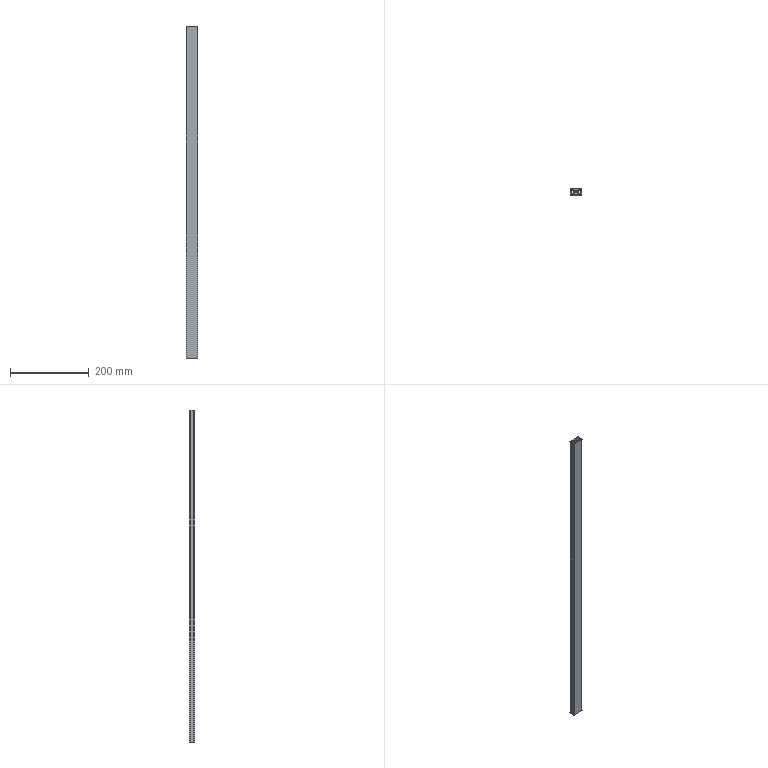Part | SolidWorks | features BaseBody 1, MoveFace 1 | 1 solid | 53 faces | box 30 x 15 x 842 mm | volume 203064 mm3 | plane 38 | cylinder 15 | commonest cylinder face diameters 1 x6 5 x5 2 x4